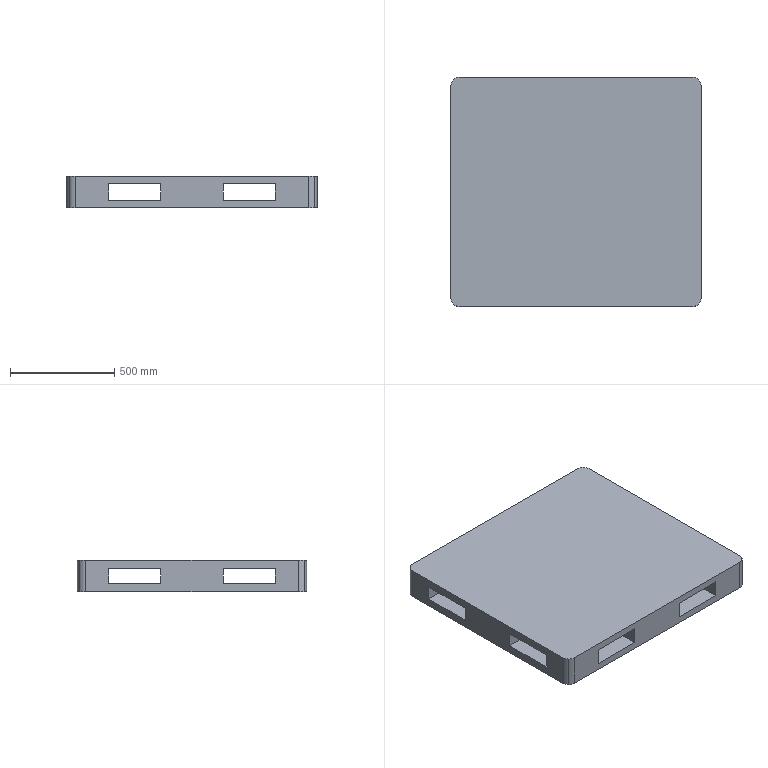Part | STEP file | PALET-1200x1100x150 | 1 solid | 46 faces | box 1200 x 1100 x 150 mm | volume 129293982 mm3 | plane 38 | cylinder 8 | commonest cylinder face diameters 80 x8